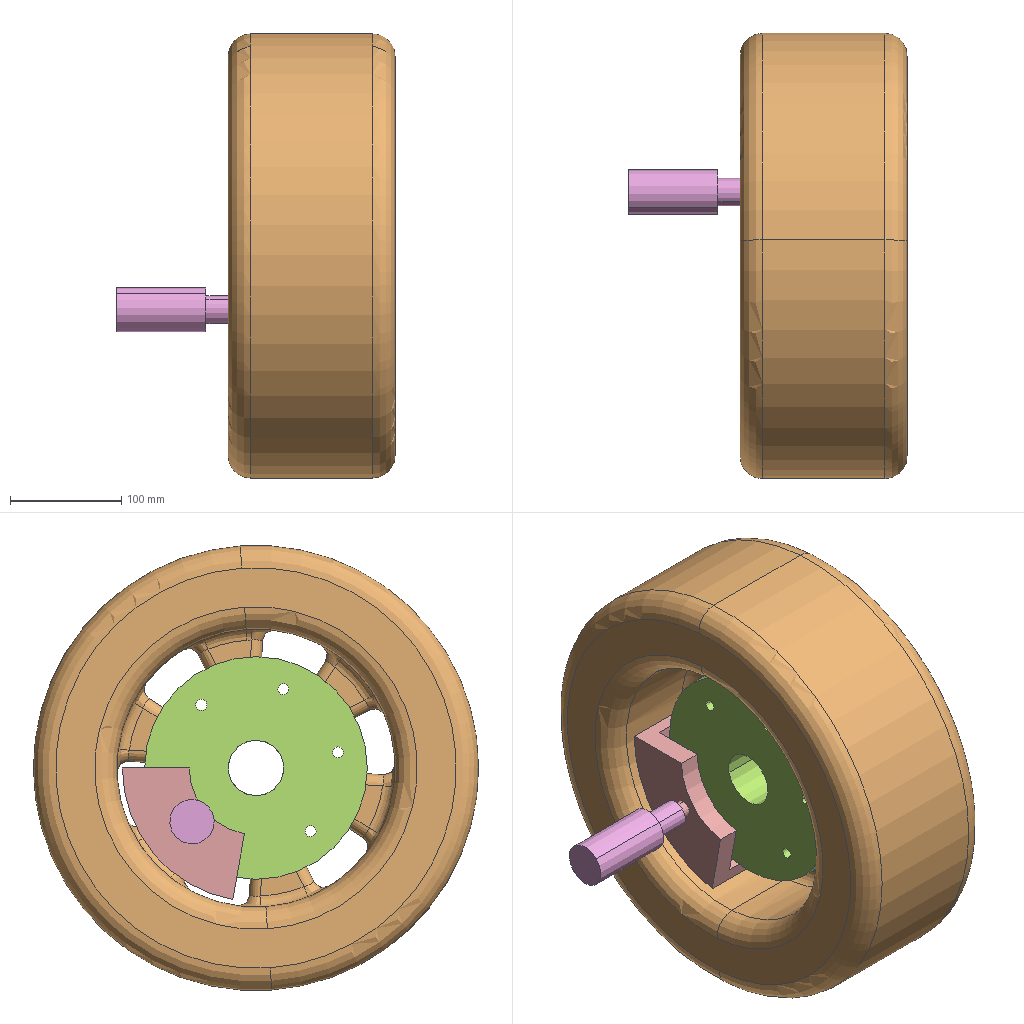Assembly | SolidWorks | 7 different items | 8 placed | box 250 x 400 x 399 mm
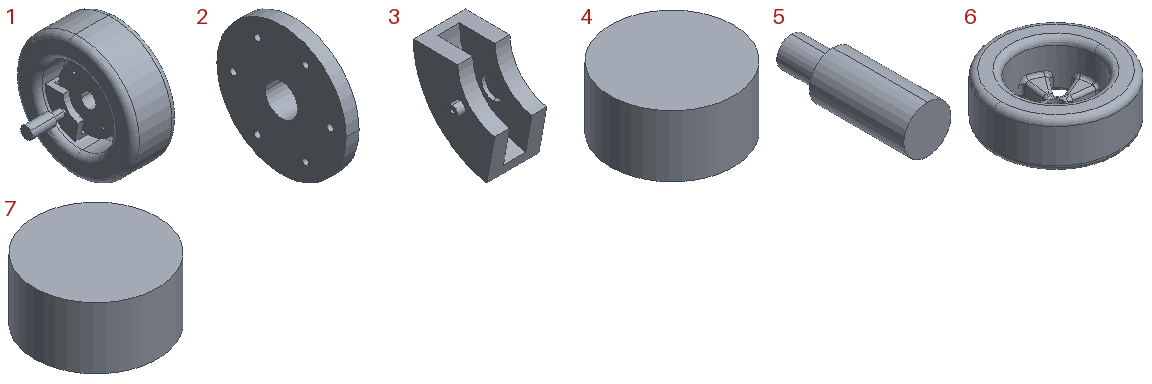Parts list (item | name | quantity | size | volume | features):
1 | (subassembly) | x1 | 250 x 400 x 400 mm | 13503610 mm3 | features AEMSimFeature 1
2 | - | x1 | 50 x 200 x 200 mm | 749898 mm3 | features CirPattern 1, Fillet 1, ICE 1, Revolution 1
3 | - | x1 | 80 x 109.581 x 118.177 mm | 225708 mm3 | features Cut 1, ICE 1, Revolution 1, Shell 1
4 | - | x1 | 30 x 30 x 15 mm | 10603 mm3 | features Extrusion 1
5 | - | x1 | 40 x 115 x 40 mm | 61163 mm3 | features Revolution 1
6 | - | x1 | 400 x 400 x 150 mm | 12435033 mm3 | features Fillet 2, ICE 2, CirPattern 1, Extrusion 1
7 | - | x2 | 30 x 30 x 15 mm | 10603 mm3 | features Extrusion 1
Mates (type | each side: item.copy, entity, surface, feature):
Concentric | 7.1 face cylinder Boss-Extrude1 | 7.2 face cylinder Boss-Extrude1
Concentric | 7.1 face cylinder Boss-Extrude1 | 3.1 face cylinder Cut-Extrude1
Concentric | 3.1 face cylinder Revolve1 | 2.1 face cylinder Revolve1
DistanceDim | 3.1 face plane Revolve1 | 2.1 face plane Revolve1
Concentric | 3.1 face cylinder Boss-Extrude1 | 5.1 face cylinder Revolve1
Coincident | 3.1 face plane Boss-Extrude1 | 5.1 face plane Revolve1
Concentric | 5.1 face cylinder Revolve1 | 4.1 face cylinder Boss-Extrude1
Concentric | 2.1 face cylinder Revolve1 | 6.1 face cylinder Cut-Extrude1
Coincident | 2.1 face plane Revolve1 | 6.1 face plane Cut-Extrude1
Lock | 2.1 select_type:0 | 6.1 select_type:0